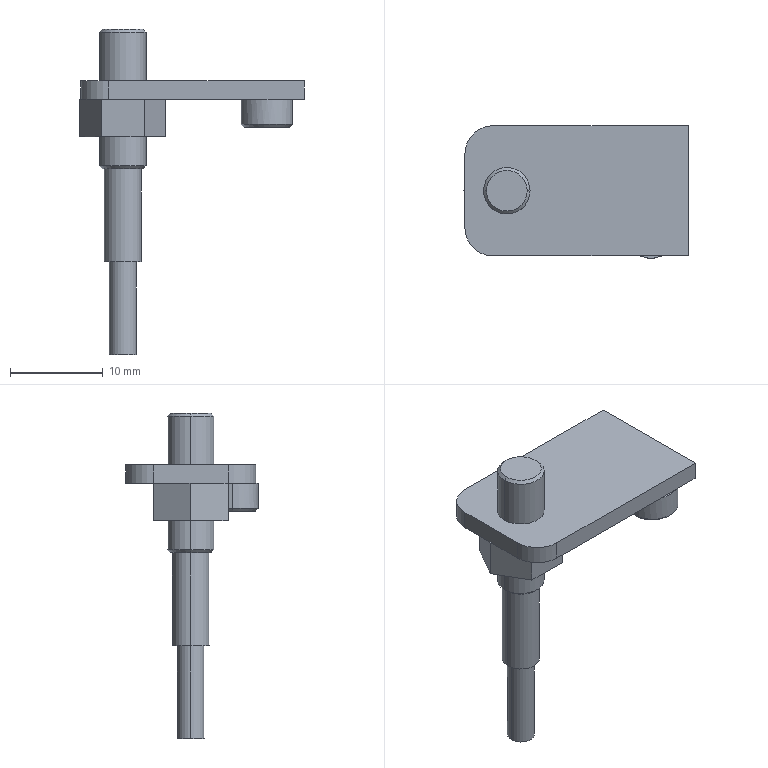Part | STEP file | 1105WWT4_1 | 1 solid | 45 faces | box 24.119 x 14.25 x 35 mm | volume 1315 mm3 | plane 27 | cylinder 12 | cone 6 | commonest cylinder face diameters 5 x4 2.9 x2 4 x2 5.5 x2 6 x2
STEP:
#1=CARTESIAN_POINT('',(-40.,-5.,-7.266));
#2=VERTEX_POINT('',#1);
#3=CARTESIAN_POINT('',(-35.,-5.,-7.266));
#4=VERTEX_POINT('',#3);
#5=CARTESIAN_POINT('',(-37.5,-5.,-7.266));
#6=DIRECTION('',(0.,0.,-1.));
#7=DIRECTION('',(-1.,0.,0.));
#8=AXIS2_PLACEMENT_3D('',#5,#6,#7);
#9=CIRCLE('',#8,2.5);
#10=EDGE_CURVE('',#2,#4,#9,.T.);
#11=ORIENTED_EDGE('',*,*,#10,.T.);
#12=CARTESIAN_POINT('',(-35.,-5.,-12.5));
#13=VERTEX_POINT('',#12);
#14=CARTESIAN_POINT('',(-35.,-5.,-14.46));
#15=DIRECTION('',(0.,0.,-1.));
#16=VECTOR('',#15,1000.);
#17=LINE('',#14,#16);
#18=EDGE_CURVE('',#4,#13,#17,.T.);
#19=ORIENTED_EDGE('',*,*,#18,.T.);
#20=CARTESIAN_POINT('',(-40.,-5.,-12.5));
#21=VERTEX_POINT('',#20);
#22=CARTESIAN_POINT('',(-37.5,-5.,-12.5));
#23=DIRECTION('',(0.,0.,-1.));
#24=DIRECTION('',(-1.,0.,0.));
#25=AXIS2_PLACEMENT_3D('',#22,#23,#24);
#26=CIRCLE('',#25,2.5);
#27=EDGE_CURVE('',#21,#13,#26,.T.);
#28=ORIENTED_EDGE('',*,*,#27,.F.);
#29=CARTESIAN_POINT('',(-40.,-5.,-14.46));
#30=DIRECTION('',(0.,0.,-1.));
#31=VECTOR('',#30,1000.);
#32=LINE('',#29,#31);
#33=EDGE_CURVE('',#2,#21,#32,.T.);
#34=ORIENTED_EDGE('',*,*,#33,.F.);
#35=EDGE_LOOP('',(#11,#19,#28,#34));
#36=FACE_OUTER_BOUND('',#35,.T.);
#37=CARTESIAN_POINT('',(-37.5,-5.,-14.46));
#38=DIRECTION('',(0.,0.,-1.));
#39=DIRECTION('',(-1.,0.,0.));
#40=AXIS2_PLACEMENT_3D('',#37,#38,#39);
#41=CYLINDRICAL_SURFACE('',#40,2.5);
#42=ADVANCED_FACE('',(#36),#41,.T.);
#43=CARTESIAN_POINT('',(-39.693,-5.,-6.96));
#44=VERTEX_POINT('',#43);
#45=CARTESIAN_POINT('',(-35.307,-5.,-6.96));
#46=VERTEX_POINT('',#45);
#47=CARTESIAN_POINT('',(-37.5,-5.,-6.96));
#48=DIRECTION('',(0.,0.,-1.));
#49=DIRECTION('',(-1.,0.,0.));
#50=AXIS2_PLACEMENT_3D('',#47,#48,#49);
#51=CIRCLE('',#50,2.193);
#52=EDGE_CURVE('',#44,#46,#51,.T.);
#53=ORIENTED_EDGE('',*,*,#52,.T.);
#54=CARTESIAN_POINT('',(-35.,-5.,-7.267));
#55=DIRECTION('',(0.7071,0.,-0.7071));
#56=VECTOR('',#55,1000.);
#57=LINE('',#54,#56);
#58=EDGE_CURVE('',#46,#4,#57,.T.);
#59=ORIENTED_EDGE('',*,*,#58,.T.);
#60=ORIENTED_EDGE('',*,*,#10,.F.);
#61=CARTESIAN_POINT('',(-40.,-5.,-7.267));
#62=DIRECTION('',(-0.7071,0.,-0.7071));
#63=VECTOR('',#62,1000.);
#64=LINE('',#61,#63);
#65=EDGE_CURVE('',#44,#2,#64,.T.);
#66=ORIENTED_EDGE('',*,*,#65,.F.);
#67=EDGE_LOOP('',(#53,#59,#60,#66));
#68=FACE_OUTER_BOUND('',#67,.T.);
#69=CARTESIAN_POINT('',(-37.5,-5.,-7.267));
#70=DIRECTION('',(0.,0.,-1.));
#71=DIRECTION('',(-1.,0.,0.));
#72=AXIS2_PLACEMENT_3D('',#69,#70,#71);
#73=CONICAL_SURFACE('',#72,2.5,0.7854);
#74=ADVANCED_FACE('',(#68),#73,.T.);
#75=CARTESIAN_POINT('',(-19.25,-9.5,-17.2));
#76=VERTEX_POINT('',#75);
#77=CARTESIAN_POINT('',(-24.75,-9.5,-17.2));
#78=VERTEX_POINT('',#77);
#79=CARTESIAN_POINT('',(-22.,-9.5,-17.2));
#80=DIRECTION('',(0.,0.,1.));
#81=DIRECTION('',(1.,0.,0.));
#82=AXIS2_PLACEMENT_3D('',#79,#80,#81);
#83=CIRCLE('',#82,2.75);
#84=EDGE_CURVE('',#76,#78,#83,.T.);
#85=ORIENTED_EDGE('',*,*,#84,.T.);
#86=CARTESIAN_POINT('',(-24.75,-9.5,-14.5));
#87=VERTEX_POINT('',#86);
#88=CARTESIAN_POINT('',(-24.75,-9.5,-15.85));
#89=DIRECTION('',(0.,0.,1.));
#90=VECTOR('',#89,1000.);
#91=LINE('',#88,#90);
#92=EDGE_CURVE('',#78,#87,#91,.T.);
#93=ORIENTED_EDGE('',*,*,#92,.T.);
#94=CARTESIAN_POINT('',(-19.25,-9.5,-14.5));
#95=VERTEX_POINT('',#94);
#96=CARTESIAN_POINT('',(-22.,-9.5,-14.5));
#97=DIRECTION('',(0.,0.,-1.));
#98=DIRECTION('',(1.,0.,0.));
#99=AXIS2_PLACEMENT_3D('',#96,#97,#98);
#100=CIRCLE('',#99,2.75);
#101=EDGE_CURVE('',#87,#95,#100,.T.);
#102=ORIENTED_EDGE('',*,*,#101,.T.);
#103=CARTESIAN_POINT('',(-19.25,-9.5,-15.85));
#104=DIRECTION('',(0.,0.,1.));
#105=VECTOR('',#104,1000.);
#106=LINE('',#103,#105);
#107=EDGE_CURVE('',#76,#95,#106,.T.);
#108=ORIENTED_EDGE('',*,*,#107,.F.);
#109=EDGE_LOOP('',(#85,#93,#102,#108));
#110=FACE_OUTER_BOUND('',#109,.T.);
#111=CARTESIAN_POINT('',(-22.,-9.5,-15.85));
#112=DIRECTION('',(0.,0.,1.));
#113=DIRECTION('',(1.,0.,0.));
#114=AXIS2_PLACEMENT_3D('',#111,#112,#113);
#115=CYLINDRICAL_SURFACE('',#114,2.75);
#116=ADVANCED_FACE('',(#110),#115,.T.);
#117=CARTESIAN_POINT('',(-19.55,-9.5,-17.5));
#118=VERTEX_POINT('',#117);
#119=CARTESIAN_POINT('',(-24.45,-9.5,-17.5));
#120=VERTEX_POINT('',#119);
#121=CARTESIAN_POINT('',(-22.,-9.5,-17.5));
#122=DIRECTION('',(0.,0.,1.));
#123=DIRECTION('',(1.,0.,0.));
#124=AXIS2_PLACEMENT_3D('',#121,#122,#123);
#125=CIRCLE('',#124,2.45);
#126=EDGE_CURVE('',#118,#120,#125,.T.);
#127=ORIENTED_EDGE('',*,*,#126,.T.);
#128=CARTESIAN_POINT('',(-24.75,-9.5,-17.2));
#129=DIRECTION('',(-0.7071,0.,0.7071));
#130=VECTOR('',#129,1000.);
#131=LINE('',#128,#130);
#132=EDGE_CURVE('',#120,#78,#131,.T.);
#133=ORIENTED_EDGE('',*,*,#132,.T.);
#134=ORIENTED_EDGE('',*,*,#84,.F.);
#135=CARTESIAN_POINT('',(-19.25,-9.5,-17.2));
#136=DIRECTION('',(0.7071,0.,0.7071));
#137=VECTOR('',#136,1000.);
#138=LINE('',#135,#137);
#139=EDGE_CURVE('',#118,#76,#138,.T.);
#140=ORIENTED_EDGE('',*,*,#139,.F.);
#141=EDGE_LOOP('',(#127,#133,#134,#140));
#142=FACE_OUTER_BOUND('',#141,.T.);
#143=CARTESIAN_POINT('',(-22.,-9.5,-17.2));
#144=DIRECTION('',(0.,0.,1.));
#145=DIRECTION('',(1.,0.,0.));
#146=AXIS2_PLACEMENT_3D('',#143,#144,#145);
#147=CONICAL_SURFACE('',#146,2.75,0.7854);
#148=ADVANCED_FACE('',(#142),#147,.T.);
#149=CARTESIAN_POINT('',(-40.,-5.,-18.5));
#150=VERTEX_POINT('',#149);
#151=CARTESIAN_POINT('',(-35.,-5.,-18.5));
#152=VERTEX_POINT('',#151);
#153=CARTESIAN_POINT('',(-37.5,-5.,-18.5));
#154=DIRECTION('',(0.,0.,-1.));
#155=DIRECTION('',(-1.,0.,0.));
#156=AXIS2_PLACEMENT_3D('',#153,#154,#155);
#157=CIRCLE('',#156,2.5);
#158=EDGE_CURVE('',#150,#152,#157,.T.);
#159=ORIENTED_EDGE('',*,*,#158,.T.);
#160=CARTESIAN_POINT('',(-35.,-5.,-21.654));
#161=VERTEX_POINT('',#160);
#162=CARTESIAN_POINT('',(-35.,-5.,-14.46));
#163=DIRECTION('',(0.,0.,-1.));
#164=VECTOR('',#163,1000.);
#165=LINE('',#162,#164);
#166=EDGE_CURVE('',#152,#161,#165,.T.);
#167=ORIENTED_EDGE('',*,*,#166,.T.);
#168=CARTESIAN_POINT('',(-40.,-5.,-21.654));
#169=VERTEX_POINT('',#168);
#170=CARTESIAN_POINT('',(-37.5,-5.,-21.654));
#171=DIRECTION('',(0.,0.,1.));
#172=DIRECTION('',(-1.,0.,0.));
#173=AXIS2_PLACEMENT_3D('',#170,#171,#172);
#174=CIRCLE('',#173,2.5);
#175=EDGE_CURVE('',#161,#169,#174,.T.);
#176=ORIENTED_EDGE('',*,*,#175,.T.);
#177=CARTESIAN_POINT('',(-40.,-5.,-14.46));
#178=DIRECTION('',(0.,0.,-1.));
#179=VECTOR('',#178,1000.);
#180=LINE('',#177,#179);
#181=EDGE_CURVE('',#150,#169,#180,.T.);
#182=ORIENTED_EDGE('',*,*,#181,.F.);
#183=EDGE_LOOP('',(#159,#167,#176,#182));
#184=FACE_OUTER_BOUND('',#183,.T.);
#185=CARTESIAN_POINT('',(-37.5,-5.,-14.46));
#186=DIRECTION('',(0.,0.,-1.));
#187=DIRECTION('',(-1.,0.,0.));
#188=AXIS2_PLACEMENT_3D('',#185,#186,#187);
#189=CYLINDRICAL_SURFACE('',#188,2.5);
#190=ADVANCED_FACE('',(#184),#189,.T.);
#191=CARTESIAN_POINT('',(-35.306,-5.,-21.96));
#192=VERTEX_POINT('',#191);
#193=CARTESIAN_POINT('',(-39.694,-5.,-21.96));
#194=VERTEX_POINT('',#193);
#195=CARTESIAN_POINT('',(-37.5,-5.,-21.96));
#196=DIRECTION('',(0.,0.,1.));
#197=DIRECTION('',(1.,0.,0.));
#198=AXIS2_PLACEMENT_3D('',#195,#196,#197);
#199=CIRCLE('',#198,2.194);
#200=EDGE_CURVE('',#192,#194,#199,.T.);
#201=ORIENTED_EDGE('',*,*,#200,.T.);
#202=CARTESIAN_POINT('',(-40.,-5.,-21.654));
#203=DIRECTION('',(-0.7071,0.,0.7071));
#204=VECTOR('',#203,1000.);
#205=LINE('',#202,#204);
#206=EDGE_CURVE('',#194,#169,#205,.T.);
#207=ORIENTED_EDGE('',*,*,#206,.T.);
#208=ORIENTED_EDGE('',*,*,#175,.F.);
#209=CARTESIAN_POINT('',(-35.,-5.,-21.654));
#210=DIRECTION('',(0.7071,0.,0.7071));
#211=VECTOR('',#210,1000.);
#212=LINE('',#209,#211);
#213=EDGE_CURVE('',#192,#161,#212,.T.);
#214=ORIENTED_EDGE('',*,*,#213,.F.);
#215=EDGE_LOOP('',(#201,#207,#208,#214));
#216=FACE_OUTER_BOUND('',#215,.T.);
#217=CARTESIAN_POINT('',(-37.5,-5.,-21.654));
#218=DIRECTION('',(0.,0.,1.));
#219=DIRECTION('',(1.,0.,0.));
#220=AXIS2_PLACEMENT_3D('',#217,#218,#219);
#221=CONICAL_SURFACE('',#220,2.5,0.7854);
#222=ADVANCED_FACE('',(#216),#221,.T.);
#223=CARTESIAN_POINT('',(-35.5,-5.,-21.96));
#224=VERTEX_POINT('',#223);
#225=CARTESIAN_POINT('',(-39.5,-5.,-21.96));
#226=VERTEX_POINT('',#225);
#227=CARTESIAN_POINT('',(-37.5,-5.,-21.96));
#228=DIRECTION('',(0.,0.,1.));
#229=DIRECTION('',(-1.,0.,0.));
#230=AXIS2_PLACEMENT_3D('',#227,#228,#229);
#231=CIRCLE('',#230,2.);
#232=EDGE_CURVE('',#224,#226,#231,.T.);
#233=ORIENTED_EDGE('',*,*,#232,.F.);
#234=CARTESIAN_POINT('',(-35.5,-5.,-31.96));
#235=VERTEX_POINT('',#234);
#236=CARTESIAN_POINT('',(-35.5,-5.,-26.96));
#237=DIRECTION('',(0.,0.,-1.));
#238=VECTOR('',#237,1000.);
#239=LINE('',#236,#238);
#240=EDGE_CURVE('',#224,#235,#239,.T.);
#241=ORIENTED_EDGE('',*,*,#240,.T.);
#242=CARTESIAN_POINT('',(-39.5,-5.,-31.96));
#243=VERTEX_POINT('',#242);
#244=CARTESIAN_POINT('',(-37.5,-5.,-31.96));
#245=DIRECTION('',(0.,0.,1.));
#246=DIRECTION('',(-1.,0.,0.));
#247=AXIS2_PLACEMENT_3D('',#244,#245,#246);
#248=CIRCLE('',#247,2.);
#249=EDGE_CURVE('',#235,#243,#248,.T.);
#250=ORIENTED_EDGE('',*,*,#249,.T.);
#251=CARTESIAN_POINT('',(-39.5,-5.,-26.96));
#252=DIRECTION('',(0.,0.,-1.));
#253=VECTOR('',#252,1000.);
#254=LINE('',#251,#253);
#255=EDGE_CURVE('',#226,#243,#254,.T.);
#256=ORIENTED_EDGE('',*,*,#255,.F.);
#257=EDGE_LOOP('',(#233,#241,#250,#256));
#258=FACE_OUTER_BOUND('',#257,.T.);
#259=CARTESIAN_POINT('',(-37.5,-5.,-26.96));
#260=DIRECTION('',(0.,0.,-1.));
#261=DIRECTION('',(-1.,0.,0.));
#262=AXIS2_PLACEMENT_3D('',#259,#260,#261);
#263=CYLINDRICAL_SURFACE('',#262,2.);
#264=ADVANCED_FACE('',(#258),#263,.T.);
#265=CARTESIAN_POINT('',(-36.05,-5.,-31.96));
#266=VERTEX_POINT('',#265);
#267=CARTESIAN_POINT('',(-38.95,-5.,-31.96));
#268=VERTEX_POINT('',#267);
#269=CARTESIAN_POINT('',(-37.5,-5.,-31.96));
#270=DIRECTION('',(0.,0.,1.));
#271=DIRECTION('',(-1.,0.,0.));
#272=AXIS2_PLACEMENT_3D('',#269,#270,#271);
#273=CIRCLE('',#272,1.45);
#274=EDGE_CURVE('',#266,#268,#273,.T.);
#275=ORIENTED_EDGE('',*,*,#274,.F.);
#276=CARTESIAN_POINT('',(-36.05,-5.,-41.96));
#277=VERTEX_POINT('',#276);
#278=CARTESIAN_POINT('',(-36.05,-5.,-36.96));
#279=DIRECTION('',(0.,0.,-1.));
#280=VECTOR('',#279,1000.);
#281=LINE('',#278,#280);
#282=EDGE_CURVE('',#266,#277,#281,.T.);
#283=ORIENTED_EDGE('',*,*,#282,.T.);
#284=CARTESIAN_POINT('',(-38.95,-5.,-41.96));
#285=VERTEX_POINT('',#284);
#286=CARTESIAN_POINT('',(-37.5,-5.,-41.96));
#287=DIRECTION('',(0.,0.,1.));
#288=DIRECTION('',(-1.,0.,0.));
#289=AXIS2_PLACEMENT_3D('',#286,#287,#288);
#290=CIRCLE('',#289,1.45);
#291=EDGE_CURVE('',#277,#285,#290,.T.);
#292=ORIENTED_EDGE('',*,*,#291,.T.);
#293=CARTESIAN_POINT('',(-38.95,-5.,-36.96));
#294=DIRECTION('',(0.,0.,-1.));
#295=VECTOR('',#294,1000.);
#296=LINE('',#293,#295);
#297=EDGE_CURVE('',#268,#285,#296,.T.);
#298=ORIENTED_EDGE('',*,*,#297,.F.);
#299=EDGE_LOOP('',(#275,#283,#292,#298));
#300=FACE_OUTER_BOUND('',#299,.T.);
#301=CARTESIAN_POINT('',(-37.5,-5.,-36.96));
#302=DIRECTION('',(0.,0.,-1.));
#303=DIRECTION('',(-1.,0.,0.));
#304=AXIS2_PLACEMENT_3D('',#301,#302,#303);
#305=CYLINDRICAL_SURFACE('',#304,1.45);
#306=ADVANCED_FACE('',(#300),#305,.T.);
#307=ORIENTED_EDGE('',*,*,#27,.T.);
#308=CARTESIAN_POINT('',(-37.5,-5.,-12.5));
#309=DIRECTION('',(0.,0.,-1.));
#310=DIRECTION('',(-1.,0.,0.));
#311=AXIS2_PLACEMENT_3D('',#308,#309,#310);
#312=CIRCLE('',#311,2.5);
#313=EDGE_CURVE('',#13,#21,#312,.T.);
#314=ORIENTED_EDGE('',*,*,#313,.T.);
#315=EDGE_LOOP('',(#307,#314));
#316=FACE_BOUND('',#315,.T.);
#317=CARTESIAN_POINT('',(-42.,-9.,-12.5));
#318=VERTEX_POINT('',#317);
#319=CARTESIAN_POINT('',(-39.,-12.,-12.5));
#320=VERTEX_POINT('',#319);
#321=CARTESIAN_POINT('',(-39.,-9.,-12.5));
#322=DIRECTION('',(0.,0.,1.));
#323=DIRECTION('',(1.,0.,0.));
#324=AXIS2_PLACEMENT_3D('',#321,#322,#323);
#325=CIRCLE('',#324,3.);
#326=EDGE_CURVE('',#318,#320,#325,.T.);
#327=ORIENTED_EDGE('',*,*,#326,.T.);
#328=CARTESIAN_POINT('',(-18.,-12.,-12.5));
#329=VERTEX_POINT('',#328);
#330=CARTESIAN_POINT('',(-37.5,-12.,-12.5));
#331=DIRECTION('',(1.,0.,0.));
#332=VECTOR('',#331,1000.);
#333=LINE('',#330,#332);
#334=EDGE_CURVE('',#320,#329,#333,.T.);
#335=ORIENTED_EDGE('',*,*,#334,.T.);
#336=CARTESIAN_POINT('',(-18.,2.,-12.5));
#337=VERTEX_POINT('',#336);
#338=CARTESIAN_POINT('',(-18.,-5.,-12.5));
#339=DIRECTION('',(0.,1.,0.));
#340=VECTOR('',#339,1000.);
#341=LINE('',#338,#340);
#342=EDGE_CURVE('',#329,#337,#341,.T.);
#343=ORIENTED_EDGE('',*,*,#342,.T.);
#344=CARTESIAN_POINT('',(-39.,2.,-12.5));
#345=VERTEX_POINT('',#344);
#346=CARTESIAN_POINT('',(-37.5,2.,-12.5));
#347=DIRECTION('',(-1.,0.,0.));
#348=VECTOR('',#347,1000.);
#349=LINE('',#346,#348);
#350=EDGE_CURVE('',#337,#345,#349,.T.);
#351=ORIENTED_EDGE('',*,*,#350,.T.);
#352=CARTESIAN_POINT('',(-42.,-1.,-12.5));
#353=VERTEX_POINT('',#352);
#354=CARTESIAN_POINT('',(-39.,-1.,-12.5));
#355=DIRECTION('',(0.,0.,1.));
#356=DIRECTION('',(1.,0.,0.));
#357=AXIS2_PLACEMENT_3D('',#354,#355,#356);
#358=CIRCLE('',#357,3.);
#359=EDGE_CURVE('',#345,#353,#358,.T.);
#360=ORIENTED_EDGE('',*,*,#359,.T.);
#361=CARTESIAN_POINT('',(-42.,-5.,-12.5));
#362=DIRECTION('',(0.,-1.,0.));
#363=VECTOR('',#362,1000.);
#364=LINE('',#361,#363);
#365=EDGE_CURVE('',#353,#318,#364,.T.);
#366=ORIENTED_EDGE('',*,*,#365,.T.);
#367=EDGE_LOOP('',(#327,#335,#343,#351,#360,#366));
#368=FACE_OUTER_BOUND('',#367,.T.);
#369=CARTESIAN_POINT('',(-37.5,-5.,-12.5));
#370=DIRECTION('',(0.,0.,1.));
#371=DIRECTION('',(1.,0.,0.));
#372=AXIS2_PLACEMENT_3D('',#369,#370,#371);
#373=PLANE('',#372);
#374=ADVANCED_FACE('',(#316,#368),#373,.T.);
#375=ORIENTED_EDGE('',*,*,#18,.F.);
#376=CARTESIAN_POINT('',(-37.5,-5.,-7.266));
#377=DIRECTION('',(0.,0.,-1.));
#378=DIRECTION('',(-1.,0.,0.));
#379=AXIS2_PLACEMENT_3D('',#376,#377,#378);
#380=CIRCLE('',#379,2.5);
#381=EDGE_CURVE('',#4,#2,#380,.T.);
#382=ORIENTED_EDGE('',*,*,#381,.T.);
#383=ORIENTED_EDGE('',*,*,#33,.T.);
#384=ORIENTED_EDGE('',*,*,#313,.F.);
#385=EDGE_LOOP('',(#375,#382,#383,#384));
#386=FACE_OUTER_BOUND('',#385,.T.);
#387=CARTESIAN_POINT('',(-37.5,-5.,-14.46));
#388=DIRECTION('',(0.,0.,-1.));
#389=DIRECTION('',(-1.,0.,0.));
#390=AXIS2_PLACEMENT_3D('',#387,#388,#389);
#391=CYLINDRICAL_SURFACE('',#390,2.5);
#392=ADVANCED_FACE('',(#386),#391,.T.);
#393=ORIENTED_EDGE('',*,*,#334,.F.);
#394=CARTESIAN_POINT('',(-39.,-12.,-14.5));
#395=VERTEX_POINT('',#394);
#396=CARTESIAN_POINT('',(-39.,-12.,-12.5));
#397=DIRECTION('',(0.,0.,-1.));
#398=VECTOR('',#397,1000.);
#399=LINE('',#396,#398);
#400=EDGE_CURVE('',#320,#395,#399,.T.);
#401=ORIENTED_EDGE('',*,*,#400,.T.);
#402=CARTESIAN_POINT('',(-23.146,-12.,-14.5));
#403=VERTEX_POINT('',#402);
#404=CARTESIAN_POINT('',(-39.,-12.,-14.5));
#405=DIRECTION('',(1.,0.,0.));
#406=VECTOR('',#405,1000.);
#407=LINE('',#404,#406);
#408=EDGE_CURVE('',#395,#403,#407,.T.);
#409=ORIENTED_EDGE('',*,*,#408,.T.);
#410=CARTESIAN_POINT('',(-20.854,-12.,-14.5));
#411=VERTEX_POINT('',#410);
#412=CARTESIAN_POINT('',(-39.,-12.,-14.5));
#413=DIRECTION('',(1.,0.,0.));
#414=VECTOR('',#413,1000.);
#415=LINE('',#412,#414);
#416=EDGE_CURVE('',#403,#411,#415,.T.);
#417=ORIENTED_EDGE('',*,*,#416,.T.);
#418=CARTESIAN_POINT('',(-18.,-12.,-14.5));
#419=VERTEX_POINT('',#418);
#420=CARTESIAN_POINT('',(-39.,-12.,-14.5));
#421=DIRECTION('',(1.,0.,0.));
#422=VECTOR('',#421,1000.);
#423=LINE('',#420,#422);
#424=EDGE_CURVE('',#411,#419,#423,.T.);
#425=ORIENTED_EDGE('',*,*,#424,.T.);
#426=CARTESIAN_POINT('',(-18.,-12.,-12.5));
#427=DIRECTION('',(0.,0.,1.));
#428=VECTOR('',#427,1000.);
#429=LINE('',#426,#428);
#430=EDGE_CURVE('',#419,#329,#429,.T.);
#431=ORIENTED_EDGE('',*,*,#430,.T.);
#432=EDGE_LOOP('',(#393,#401,#409,#417,#425,#431));
#433=FACE_OUTER_BOUND('',#432,.T.);
#434=CARTESIAN_POINT('',(-39.,-12.,-12.5));
#435=DIRECTION('',(0.,-1.,0.));
#436=DIRECTION('',(0.,0.,-1.));
#437=AXIS2_PLACEMENT_3D('',#434,#435,#436);
#438=PLANE('',#437);
#439=ADVANCED_FACE('',(#433),#438,.T.);
#440=ORIENTED_EDGE('',*,*,#326,.F.);
#441=CARTESIAN_POINT('',(-42.,-9.,-14.5));
#442=VERTEX_POINT('',#441);
#443=CARTESIAN_POINT('',(-42.,-9.,-12.5));
#444=DIRECTION('',(0.,0.,-1.));
#445=VECTOR('',#444,1000.);
#446=LINE('',#443,#445);
#447=EDGE_CURVE('',#318,#442,#446,.T.);
#448=ORIENTED_EDGE('',*,*,#447,.T.);
#449=CARTESIAN_POINT('',(-39.,-9.,-14.5));
#450=DIRECTION('',(0.,0.,1.));
#451=DIRECTION('',(1.,0.,0.));
#452=AXIS2_PLACEMENT_3D('',#449,#450,#451);
#453=CIRCLE('',#452,3.);
#454=EDGE_CURVE('',#442,#395,#453,.T.);
#455=ORIENTED_EDGE('',*,*,#454,.T.);
#456=ORIENTED_EDGE('',*,*,#400,.F.);
#457=EDGE_LOOP('',(#440,#448,#455,#456));
#458=FACE_OUTER_BOUND('',#457,.T.);
#459=CARTESIAN_POINT('',(-39.,-9.,-12.5));
#460=DIRECTION('',(0.,0.,1.));
#461=DIRECTION('',(1.,0.,0.));
#462=AXIS2_PLACEMENT_3D('',#459,#460,#461);
#463=CYLINDRICAL_SURFACE('',#462,3.);
#464=ADVANCED_FACE('',(#458),#463,.T.);
#465=ORIENTED_EDGE('',*,*,#365,.F.);
#466=CARTESIAN_POINT('',(-42.,-1.,-14.5));
#467=VERTEX_POINT('',#466);
#468=CARTESIAN_POINT('',(-42.,-1.,-12.5));
#469=DIRECTION('',(0.,0.,-1.));
#470=VECTOR('',#469,1000.);
#471=LINE('',#468,#470);
#472=EDGE_CURVE('',#353,#467,#471,.T.);
#473=ORIENTED_EDGE('',*,*,#472,.T.);
#474=CARTESIAN_POINT('',(-42.,-4.794,-14.5));
#475=VERTEX_POINT('',#474);
#476=CARTESIAN_POINT('',(-42.,-1.,-14.5));
#477=DIRECTION('',(0.,-1.,0.));
#478=VECTOR('',#477,1000.);
#479=LINE('',#476,#478);
#480=EDGE_CURVE('',#467,#475,#479,.T.);
#481=ORIENTED_EDGE('',*,*,#480,.T.);
#482=CARTESIAN_POINT('',(-42.,-5.206,-14.5));
#483=VERTEX_POINT('',#482);
#484=CARTESIAN_POINT('',(-42.,-1.,-14.5));
#485=DIRECTION('',(0.,-1.,0.));
#486=VECTOR('',#485,1000.);
#487=LINE('',#484,#486);
#488=EDGE_CURVE('',#475,#483,#487,.T.);
#489=ORIENTED_EDGE('',*,*,#488,.T.);
#490=CARTESIAN_POINT('',(-42.,-1.,-14.5));
#491=DIRECTION('',(0.,-1.,0.));
#492=VECTOR('',#491,1000.);
#493=LINE('',#490,#492);
#494=EDGE_CURVE('',#483,#442,#493,.T.);
#495=ORIENTED_EDGE('',*,*,#494,.T.);
#496=ORIENTED_EDGE('',*,*,#447,.F.);
#497=EDGE_LOOP('',(#465,#473,#481,#489,#495,#496));
#498=FACE_OUTER_BOUND('',#497,.T.);
#499=CARTESIAN_POINT('',(-42.,-1.,-12.5));
#500=DIRECTION('',(-1.,0.,0.));
#501=DIRECTION('',(0.,0.,1.));
#502=AXIS2_PLACEMENT_3D('',#499,#500,#501);
#503=PLANE('',#502);
#504=ADVANCED_FACE('',(#498),#503,.T.);
#505=ORIENTED_EDGE('',*,*,#359,.F.);
#506=CARTESIAN_POINT('',(-39.,2.,-14.5));
#507=VERTEX_POINT('',#506);
#508=CARTESIAN_POINT('',(-39.,2.,-12.5));
#509=DIRECTION('',(0.,0.,-1.));
#510=VECTOR('',#509,1000.);
#511=LINE('',#508,#510);
#512=EDGE_CURVE('',#345,#507,#511,.T.);
#513=ORIENTED_EDGE('',*,*,#512,.T.);
#514=CARTESIAN_POINT('',(-39.,-1.,-14.5));
#515=DIRECTION('',(0.,0.,1.));
#516=DIRECTION('',(1.,0.,0.));
#517=AXIS2_PLACEMENT_3D('',#514,#515,#516);
#518=CIRCLE('',#517,3.);
#519=EDGE_CURVE('',#507,#467,#518,.T.);
#520=ORIENTED_EDGE('',*,*,#519,.T.);
#521=ORIENTED_EDGE('',*,*,#472,.F.);
#522=EDGE_LOOP('',(#505,#513,#520,#521));
#523=FACE_OUTER_BOUND('',#522,.T.);
#524=CARTESIAN_POINT('',(-39.,-1.,-12.5));
#525=DIRECTION('',(0.,0.,1.));
#526=DIRECTION('',(1.,0.,0.));
#527=AXIS2_PLACEMENT_3D('',#524,#525,#526);
#528=CYLINDRICAL_SURFACE('',#527,3.);
#529=ADVANCED_FACE('',(#523),#528,.T.);
#530=ORIENTED_EDGE('',*,*,#350,.F.);
#531=CARTESIAN_POINT('',(-18.,2.,-14.5));
#532=VERTEX_POINT('',#531);
#533=CARTESIAN_POINT('',(-18.,2.,-12.5));
#534=DIRECTION('',(0.,0.,-1.));
#535=VECTOR('',#534,1000.);
#536=LINE('',#533,#535);
#537=EDGE_CURVE('',#337,#532,#536,.T.);
#538=ORIENTED_EDGE('',*,*,#537,.T.);
#539=CARTESIAN_POINT('',(-18.,2.,-14.5));
#540=DIRECTION('',(-1.,0.,0.));
#541=VECTOR('',#540,1000.);
#542=LINE('',#539,#541);
#543=EDGE_CURVE('',#532,#507,#542,.T.);
#544=ORIENTED_EDGE('',*,*,#543,.T.);
#545=ORIENTED_EDGE('',*,*,#512,.F.);
#546=EDGE_LOOP('',(#530,#538,#544,#545));
#547=FACE_OUTER_BOUND('',#546,.T.);
#548=CARTESIAN_POINT('',(-18.,2.,-12.5));
#549=DIRECTION('',(0.,1.,0.));
#550=DIRECTION('',(0.,0.,1.));
#551=AXIS2_PLACEMENT_3D('',#548,#549,#550);
#552=PLANE('',#551);
#553=ADVANCED_FACE('',(#547),#552,.T.);
#554=ORIENTED_EDGE('',*,*,#342,.F.);
#555=ORIENTED_EDGE('',*,*,#430,.F.);
#556=CARTESIAN_POINT('',(-18.,-12.,-14.5));
#557=DIRECTION('',(0.,1.,0.));
#558=VECTOR('',#557,1000.);
#559=LINE('',#556,#558);
#560=EDGE_CURVE('',#419,#532,#559,.T.);
#561=ORIENTED_EDGE('',*,*,#560,.T.);
#562=ORIENTED_EDGE('',*,*,#537,.F.);
#563=EDGE_LOOP('',(#554,#555,#561,#562));
#564=FACE_OUTER_BOUND('',#563,.T.);
#565=CARTESIAN_POINT('',(-18.,-12.,-12.5));
#566=DIRECTION('',(1.,0.,0.));
#567=DIRECTION('',(0.,0.,-1.));
#568=AXIS2_PLACEMENT_3D('',#565,#566,#567);
#569=PLANE('',#568);
#570=ADVANCED_FACE('',(#564),#569,.T.);
#571=ORIENTED_EDGE('',*,*,#58,.F.);
#572=CARTESIAN_POINT('',(-37.5,-5.,-6.96));
#573=DIRECTION('',(0.,0.,-1.));
#574=DIRECTION('',(-1.,0.,0.));
#575=AXIS2_PLACEMENT_3D('',#572,#573,#574);
#576=CIRCLE('',#575,2.193);
#577=EDGE_CURVE('',#46,#44,#576,.T.);
#578=ORIENTED_EDGE('',*,*,#577,.T.);
#579=ORIENTED_EDGE('',*,*,#65,.T.);
#580=ORIENTED_EDGE('',*,*,#381,.F.);
#581=EDGE_LOOP('',(#571,#578,#579,#580));
#582=FACE_OUTER_BOUND('',#581,.T.);
#583=CARTESIAN_POINT('',(-37.5,-5.,-7.267));
#584=DIRECTION('',(0.,0.,-1.));
#585=DIRECTION('',(-1.,0.,0.));
#586=AXIS2_PLACEMENT_3D('',#583,#584,#585);
#587=CONICAL_SURFACE('',#586,2.5,0.7854);
#588=ADVANCED_FACE('',(#582),#587,.T.);
#589=CARTESIAN_POINT('',(-22.,-9.5,-14.5));
#590=DIRECTION('',(0.,0.,-1.));
#591=DIRECTION('',(1.,0.,0.));
#592=AXIS2_PLACEMENT_3D('',#589,#590,#591);
#593=CIRCLE('',#592,2.75);
#594=EDGE_CURVE('',#403,#87,#593,.T.);
#595=ORIENTED_EDGE('',*,*,#594,.F.);
#596=ORIENTED_EDGE('',*,*,#408,.F.);
#597=ORIENTED_EDGE('',*,*,#454,.F.);
#598=ORIENTED_EDGE('',*,*,#494,.F.);
#599=CARTESIAN_POINT('',(-39.809,-9.,-14.5));
#600=VERTEX_POINT('',#599);
#601=CARTESIAN_POINT('',(-39.809,-9.,-14.5));
#602=DIRECTION('',(-0.5,0.866,0.));
#603=VECTOR('',#602,1000.);
#604=LINE('',#601,#603);
#605=EDGE_CURVE('',#600,#483,#604,.T.);
#606=ORIENTED_EDGE('',*,*,#605,.F.);
#607=CARTESIAN_POINT('',(-35.191,-9.,-14.5));
#608=VERTEX_POINT('',#607);
#609=CARTESIAN_POINT('',(-37.5,-9.,-14.5));
#610=DIRECTION('',(-1.,0.,0.));
#611=VECTOR('',#610,1000.);
#612=LINE('',#609,#611);
#613=EDGE_CURVE('',#608,#600,#612,.T.);
#614=ORIENTED_EDGE('',*,*,#613,.F.);
#615=CARTESIAN_POINT('',(-32.881,-5.,-14.5));
#616=VERTEX_POINT('',#615);
#617=CARTESIAN_POINT('',(-32.881,-5.,-14.5));
#618=DIRECTION('',(-0.5,-0.866,0.));
#619=VECTOR('',#618,1000.);
#620=LINE('',#617,#619);
#621=EDGE_CURVE('',#616,#608,#620,.T.);
#622=ORIENTED_EDGE('',*,*,#621,.F.);
#623=CARTESIAN_POINT('',(-35.191,-1.,-14.5));
#624=VERTEX_POINT('',#623);
#625=CARTESIAN_POINT('',(-35.191,-1.,-14.5));
#626=DIRECTION('',(0.5,-0.866,0.));
#627=VECTOR('',#626,1000.);
#628=LINE('',#625,#627);
#629=EDGE_CURVE('',#624,#616,#628,.T.);
#630=ORIENTED_EDGE('',*,*,#629,.F.);
#631=CARTESIAN_POINT('',(-39.809,-1.,-14.5));
#632=VERTEX_POINT('',#631);
#633=CARTESIAN_POINT('',(-37.5,-1.,-14.5));
#634=DIRECTION('',(1.,0.,0.));
#635=VECTOR('',#634,1000.);
#636=LINE('',#633,#635);
#637=EDGE_CURVE('',#632,#624,#636,.T.);
#638=ORIENTED_EDGE('',*,*,#637,.F.);
#639=CARTESIAN_POINT('',(-42.,-4.794,-14.5));
#640=DIRECTION('',(0.5,0.866,0.));
#641=VECTOR('',#640,1000.);
#642=LINE('',#639,#641);
#643=EDGE_CURVE('',#475,#632,#642,.T.);
#644=ORIENTED_EDGE('',*,*,#643,.F.);
#645=ORIENTED_EDGE('',*,*,#480,.F.);
#646=ORIENTED_EDGE('',*,*,#519,.F.);
#647=ORIENTED_EDGE('',*,*,#543,.F.);
#648=ORIENTED_EDGE('',*,*,#560,.F.);
#649=ORIENTED_EDGE('',*,*,#424,.F.);
#650=CARTESIAN_POINT('',(-22.,-9.5,-14.5));
#651=DIRECTION('',(0.,0.,-1.));
#652=DIRECTION('',(1.,0.,0.));
#653=AXIS2_PLACEMENT_3D('',#650,#651,#652);
#654=CIRCLE('',#653,2.75);
#655=EDGE_CURVE('',#95,#411,#654,.T.);
#656=ORIENTED_EDGE('',*,*,#655,.F.);
#657=ORIENTED_EDGE('',*,*,#101,.F.);
#658=EDGE_LOOP('',(#595,#596,#597,#598,#606,#614,#622,#630,#638,#644,#645,#646,#647,#648,#649,#656,#657));
#659=FACE_OUTER_BOUND('',#658,.T.);
#660=CARTESIAN_POINT('',(-37.5,-5.,-14.5));
#661=DIRECTION('',(0.,0.,1.));
#662=DIRECTION('',(1.,0.,0.));
#663=AXIS2_PLACEMENT_3D('',#660,#661,#662);
#664=PLANE('',#663);
#665=ADVANCED_FACE('',(#659),#664,.F.);
#666=ORIENTED_EDGE('',*,*,#416,.F.);
#667=CARTESIAN_POINT('',(-22.,-9.5,-14.5));
#668=DIRECTION('',(0.,0.,1.));
#669=DIRECTION('',(1.,0.,0.));
#670=AXIS2_PLACEMENT_3D('',#667,#668,#669);
#671=CIRCLE('',#670,2.75);
#672=EDGE_CURVE('',#403,#411,#671,.T.);
#673=ORIENTED_EDGE('',*,*,#672,.T.);
#674=EDGE_LOOP('',(#666,#673));
#675=FACE_OUTER_BOUND('',#674,.T.);
#676=CARTESIAN_POINT('',(-20.625,-9.5,-14.5));
#677=DIRECTION('',(0.,0.,1.));
#678=DIRECTION('',(1.,0.,0.));
#679=AXIS2_PLACEMENT_3D('',#676,#677,#678);
#680=PLANE('',#679);
#681=ADVANCED_FACE('',(#675),#680,.T.);
#682=CARTESIAN_POINT('',(-42.119,-5.,-14.5));
#683=VERTEX_POINT('',#682);
#684=CARTESIAN_POINT('',(-42.,-4.794,-14.5));
#685=DIRECTION('',(-0.5,-0.866,0.));
#686=VECTOR('',#685,1000.);
#687=LINE('',#684,#686);
#688=EDGE_CURVE('',#475,#683,#687,.T.);
#689=ORIENTED_EDGE('',*,*,#688,.T.);
#690=CARTESIAN_POINT('',(-42.119,-5.,-14.5));
#691=DIRECTION('',(0.5,-0.866,0.));
#692=VECTOR('',#691,1000.);
#693=LINE('',#690,#692);
#694=EDGE_CURVE('',#683,#483,#693,.T.);
#695=ORIENTED_EDGE('',*,*,#694,.T.);
#696=ORIENTED_EDGE('',*,*,#488,.F.);
#697=EDGE_LOOP('',(#689,#695,#696));
#698=FACE_OUTER_BOUND('',#697,.T.);
#699=CARTESIAN_POINT('',(-37.5,-5.,-14.5));
#700=DIRECTION('',(0.,0.,1.));
#701=DIRECTION('',(1.,0.,0.));
#702=AXIS2_PLACEMENT_3D('',#699,#700,#701);
#703=PLANE('',#702);
#704=ADVANCED_FACE('',(#698),#703,.T.);
#705=ORIENTED_EDGE('',*,*,#52,.F.);
#706=ORIENTED_EDGE('',*,*,#577,.F.);
#707=EDGE_LOOP('',(#705,#706));
#708=FACE_OUTER_BOUND('',#707,.T.);
#709=CARTESIAN_POINT('',(-38.597,-5.,-6.96));
#710=DIRECTION('',(0.,0.,1.));
#711=DIRECTION('',(1.,0.,0.));
#712=AXIS2_PLACEMENT_3D('',#709,#710,#711);
#713=PLANE('',#712);
#714=ADVANCED_FACE('',(#708),#713,.T.);
#715=ORIENTED_EDGE('',*,*,#92,.F.);
#716=CARTESIAN_POINT('',(-22.,-9.5,-17.2));
#717=DIRECTION('',(0.,0.,1.));
#718=DIRECTION('',(1.,0.,0.));
#719=AXIS2_PLACEMENT_3D('',#716,#717,#718);
#720=CIRCLE('',#719,2.75);
#721=EDGE_CURVE('',#78,#76,#720,.T.);
#722=ORIENTED_EDGE('',*,*,#721,.T.);
#723=ORIENTED_EDGE('',*,*,#107,.T.);
#724=ORIENTED_EDGE('',*,*,#655,.T.);
#725=ORIENTED_EDGE('',*,*,#672,.F.);
#726=ORIENTED_EDGE('',*,*,#594,.T.);
#727=EDGE_LOOP('',(#715,#722,#723,#724,#725,#726));
#728=FACE_OUTER_BOUND('',#727,.T.);
#729=CARTESIAN_POINT('',(-22.,-9.5,-15.85));
#730=DIRECTION('',(0.,0.,1.));
#731=DIRECTION('',(1.,0.,0.));
#732=AXIS2_PLACEMENT_3D('',#729,#730,#731);
#733=CYLINDRICAL_SURFACE('',#732,2.75);
#734=ADVANCED_FACE('',(#728),#733,.T.);
#735=ORIENTED_EDGE('',*,*,#694,.F.);
#736=CARTESIAN_POINT('',(-42.119,-5.,-18.5));
#737=VERTEX_POINT('',#736);
#738=CARTESIAN_POINT('',(-42.119,-5.,-14.5));
#739=DIRECTION('',(0.,0.,-1.));
#740=VECTOR('',#739,1000.);
#741=LINE('',#738,#740);
#742=EDGE_CURVE('',#683,#737,#741,.T.);
#743=ORIENTED_EDGE('',*,*,#742,.T.);
#744=CARTESIAN_POINT('',(-39.809,-9.,-18.5));
#745=VERTEX_POINT('',#744);
#746=CARTESIAN_POINT('',(-42.119,-5.,-18.5));
#747=DIRECTION('',(0.5,-0.866,0.));
#748=VECTOR('',#747,1000.);
#749=LINE('',#746,#748);
#750=EDGE_CURVE('',#737,#745,#749,.T.);
#751=ORIENTED_EDGE('',*,*,#750,.T.);
#752=CARTESIAN_POINT('',(-39.809,-9.,-14.5));
#753=DIRECTION('',(0.,0.,1.));
#754=VECTOR('',#753,1000.);
#755=LINE('',#752,#754);
#756=EDGE_CURVE('',#745,#600,#755,.T.);
#757=ORIENTED_EDGE('',*,*,#756,.T.);
#758=ORIENTED_EDGE('',*,*,#605,.T.);
#759=EDGE_LOOP('',(#735,#743,#751,#757,#758));
#760=FACE_OUTER_BOUND('',#759,.T.);
#761=CARTESIAN_POINT('',(-42.119,-5.,-14.5));
#762=DIRECTION('',(-0.866,-0.5,0.));
#763=DIRECTION('',(0.5,-0.866,0.));
#764=AXIS2_PLACEMENT_3D('',#761,#762,#763);
#765=PLANE('',#764);
#766=ADVANCED_FACE('',(#760),#765,.T.);
#767=ORIENTED_EDGE('',*,*,#613,.T.);
#768=ORIENTED_EDGE('',*,*,#756,.F.);
#769=CARTESIAN_POINT('',(-35.191,-9.,-18.5));
#770=VERTEX_POINT('',#769);
#771=CARTESIAN_POINT('',(-39.809,-9.,-18.5));
#772=DIRECTION('',(1.,0.,0.));
#773=VECTOR('',#772,1000.);
#774=LINE('',#771,#773);
#775=EDGE_CURVE('',#745,#770,#774,.T.);
#776=ORIENTED_EDGE('',*,*,#775,.T.);
#777=CARTESIAN_POINT('',(-35.191,-9.,-14.5));
#778=DIRECTION('',(0.,0.,1.));
#779=VECTOR('',#778,1000.);
#780=LINE('',#777,#779);
#781=EDGE_CURVE('',#770,#608,#780,.T.);
#782=ORIENTED_EDGE('',*,*,#781,.T.);
#783=EDGE_LOOP('',(#767,#768,#776,#782));
#784=FACE_OUTER_BOUND('',#783,.T.);
#785=CARTESIAN_POINT('',(-39.809,-9.,-14.5));
#786=DIRECTION('',(0.,-1.,0.));
#787=DIRECTION('',(0.,0.,-1.));
#788=AXIS2_PLACEMENT_3D('',#785,#786,#787);
#789=PLANE('',#788);
#790=ADVANCED_FACE('',(#784),#789,.T.);
#791=ORIENTED_EDGE('',*,*,#621,.T.);
#792=ORIENTED_EDGE('',*,*,#781,.F.);
#793=CARTESIAN_POINT('',(-32.881,-5.,-18.5));
#794=VERTEX_POINT('',#793);
#795=CARTESIAN_POINT('',(-35.191,-9.,-18.5));
#796=DIRECTION('',(0.5,0.866,0.));
#797=VECTOR('',#796,1000.);
#798=LINE('',#795,#797);
#799=EDGE_CURVE('',#770,#794,#798,.T.);
#800=ORIENTED_EDGE('',*,*,#799,.T.);
#801=CARTESIAN_POINT('',(-32.881,-5.,-14.5));
#802=DIRECTION('',(0.,0.,1.));
#803=VECTOR('',#802,1000.);
#804=LINE('',#801,#803);
#805=EDGE_CURVE('',#794,#616,#804,.T.);
#806=ORIENTED_EDGE('',*,*,#805,.T.);
#807=EDGE_LOOP('',(#791,#792,#800,#806));
#808=FACE_OUTER_BOUND('',#807,.T.);
#809=CARTESIAN_POINT('',(-35.191,-9.,-14.5));
#810=DIRECTION('',(0.866,-0.5,0.));
#811=DIRECTION('',(0.5,0.866,0.));
#812=AXIS2_PLACEMENT_3D('',#809,#810,#811);
#813=PLANE('',#812);
#814=ADVANCED_FACE('',(#808),#813,.T.);
#815=ORIENTED_EDGE('',*,*,#629,.T.);
#816=ORIENTED_EDGE('',*,*,#805,.F.);
#817=CARTESIAN_POINT('',(-35.191,-1.,-18.5));
#818=VERTEX_POINT('',#817);
#819=CARTESIAN_POINT('',(-32.881,-5.,-18.5));
#820=DIRECTION('',(-0.5,0.866,0.));
#821=VECTOR('',#820,1000.);
#822=LINE('',#819,#821);
#823=EDGE_CURVE('',#794,#818,#822,.T.);
#824=ORIENTED_EDGE('',*,*,#823,.T.);
#825=CARTESIAN_POINT('',(-35.191,-1.,-14.5));
#826=DIRECTION('',(0.,0.,1.));
#827=VECTOR('',#826,1000.);
#828=LINE('',#825,#827);
#829=EDGE_CURVE('',#818,#624,#828,.T.);
#830=ORIENTED_EDGE('',*,*,#829,.T.);
#831=EDGE_LOOP('',(#815,#816,#824,#830));
#832=FACE_OUTER_BOUND('',#831,.T.);
#833=CARTESIAN_POINT('',(-32.881,-5.,-14.5));
#834=DIRECTION('',(0.866,0.5,0.));
#835=DIRECTION('',(-0.5,0.866,0.));
#836=AXIS2_PLACEMENT_3D('',#833,#834,#835);
#837=PLANE('',#836);
#838=ADVANCED_FACE('',(#832),#837,.T.);
#839=ORIENTED_EDGE('',*,*,#637,.T.);
#840=ORIENTED_EDGE('',*,*,#829,.F.);
#841=CARTESIAN_POINT('',(-39.809,-1.,-18.5));
#842=VERTEX_POINT('',#841);
#843=CARTESIAN_POINT('',(-35.191,-1.,-18.5));
#844=DIRECTION('',(-1.,0.,0.));
#845=VECTOR('',#844,1000.);
#846=LINE('',#843,#845);
#847=EDGE_CURVE('',#818,#842,#846,.T.);
#848=ORIENTED_EDGE('',*,*,#847,.T.);
#849=CARTESIAN_POINT('',(-39.809,-1.,-14.5));
#850=DIRECTION('',(0.,0.,1.));
#851=VECTOR('',#850,1000.);
#852=LINE('',#849,#851);
#853=EDGE_CURVE('',#842,#632,#852,.T.);
#854=ORIENTED_EDGE('',*,*,#853,.T.);
#855=EDGE_LOOP('',(#839,#840,#848,#854));
#856=FACE_OUTER_BOUND('',#855,.T.);
#857=CARTESIAN_POINT('',(-35.191,-1.,-14.5));
#858=DIRECTION('',(0.,1.,0.));
#859=DIRECTION('',(0.,0.,1.));
#860=AXIS2_PLACEMENT_3D('',#857,#858,#859);
#861=PLANE('',#860);
#862=ADVANCED_FACE('',(#856),#861,.T.);
#863=ORIENTED_EDGE('',*,*,#643,.T.);
#864=ORIENTED_EDGE('',*,*,#853,.F.);
#865=CARTESIAN_POINT('',(-39.809,-1.,-18.5));
#866=DIRECTION('',(-0.5,-0.866,0.));
#867=VECTOR('',#866,1000.);
#868=LINE('',#865,#867);
#869=EDGE_CURVE('',#842,#737,#868,.T.);
#870=ORIENTED_EDGE('',*,*,#869,.T.);
#871=ORIENTED_EDGE('',*,*,#742,.F.);
#872=ORIENTED_EDGE('',*,*,#688,.F.);
#873=EDGE_LOOP('',(#863,#864,#870,#871,#872));
#874=FACE_OUTER_BOUND('',#873,.T.);
#875=CARTESIAN_POINT('',(-39.809,-1.,-14.5));
#876=DIRECTION('',(-0.866,0.5,0.));
#877=DIRECTION('',(-0.5,-0.866,0.));
#878=AXIS2_PLACEMENT_3D('',#875,#876,#877);
#879=PLANE('',#878);
#880=ADVANCED_FACE('',(#874),#879,.T.);
#881=ORIENTED_EDGE('',*,*,#132,.F.);
#882=CARTESIAN_POINT('',(-22.,-9.5,-17.5));
#883=DIRECTION('',(0.,0.,1.));
#884=DIRECTION('',(1.,0.,0.));
#885=AXIS2_PLACEMENT_3D('',#882,#883,#884);
#886=CIRCLE('',#885,2.45);
#887=EDGE_CURVE('',#120,#118,#886,.T.);
#888=ORIENTED_EDGE('',*,*,#887,.T.);
#889=ORIENTED_EDGE('',*,*,#139,.T.);
#890=ORIENTED_EDGE('',*,*,#721,.F.);
#891=EDGE_LOOP('',(#881,#888,#889,#890));
#892=FACE_OUTER_BOUND('',#891,.T.);
#893=CARTESIAN_POINT('',(-22.,-9.5,-17.2));
#894=DIRECTION('',(0.,0.,1.));
#895=DIRECTION('',(1.,0.,0.));
#896=AXIS2_PLACEMENT_3D('',#893,#894,#895);
#897=CONICAL_SURFACE('',#896,2.75,0.7854);
#898=ADVANCED_FACE('',(#892),#897,.T.);
#899=ORIENTED_EDGE('',*,*,#158,.F.);
#900=CARTESIAN_POINT('',(-37.5,-5.,-18.5));
#901=DIRECTION('',(0.,0.,-1.));
#902=DIRECTION('',(-1.,0.,0.));
#903=AXIS2_PLACEMENT_3D('',#900,#901,#902);
#904=CIRCLE('',#903,2.5);
#905=EDGE_CURVE('',#152,#150,#904,.T.);
#906=ORIENTED_EDGE('',*,*,#905,.F.);
#907=EDGE_LOOP('',(#899,#906));
#908=FACE_BOUND('',#907,.T.);
#909=ORIENTED_EDGE('',*,*,#775,.F.);
#910=ORIENTED_EDGE('',*,*,#750,.F.);
#911=ORIENTED_EDGE('',*,*,#869,.F.);
#912=ORIENTED_EDGE('',*,*,#847,.F.);
#913=ORIENTED_EDGE('',*,*,#823,.F.);
#914=ORIENTED_EDGE('',*,*,#799,.F.);
#915=EDGE_LOOP('',(#909,#910,#911,#912,#913,#914));
#916=FACE_OUTER_BOUND('',#915,.T.);
#917=CARTESIAN_POINT('',(-37.5,-5.,-18.5));
#918=DIRECTION('',(0.,0.,1.));
#919=DIRECTION('',(1.,0.,0.));
#920=AXIS2_PLACEMENT_3D('',#917,#918,#919);
#921=PLANE('',#920);
#922=ADVANCED_FACE('',(#908,#916),#921,.F.);
#923=ORIENTED_EDGE('',*,*,#126,.F.);
#924=ORIENTED_EDGE('',*,*,#887,.F.);
#925=EDGE_LOOP('',(#923,#924));
#926=FACE_OUTER_BOUND('',#925,.T.);
#927=CARTESIAN_POINT('',(-21.278,-8.25,-17.5));
#928=VERTEX_POINT('',#927);
#929=CARTESIAN_POINT('',(-22.722,-8.25,-17.5));
#930=VERTEX_POINT('',#929);
#931=CARTESIAN_POINT('',(-20.775,-8.25,-17.5));
#932=DIRECTION('',(-1.,0.,0.));
#933=VECTOR('',#932,1000.);
#934=LINE('',#931,#933);
#935=EDGE_CURVE('',#928,#930,#934,.T.);
#936=ORIENTED_EDGE('',*,*,#935,.T.);
#937=CARTESIAN_POINT('',(-23.443,-9.5,-17.5));
#938=VERTEX_POINT('',#937);
#939=CARTESIAN_POINT('',(-22.722,-8.25,-17.5));
#940=DIRECTION('',(-0.5,-0.866,0.));
#941=VECTOR('',#940,1000.);
#942=LINE('',#939,#941);
#943=EDGE_CURVE('',#930,#938,#942,.T.);
#944=ORIENTED_EDGE('',*,*,#943,.T.);
#945=CARTESIAN_POINT('',(-22.722,-10.75,-17.5));
#946=VERTEX_POINT('',#945);
#947=CARTESIAN_POINT('',(-23.443,-9.5,-17.5));
#948=DIRECTION('',(0.5,-0.866,0.));
#949=VECTOR('',#948,1000.);
#950=LINE('',#947,#949);
#951=EDGE_CURVE('',#938,#946,#950,.T.);
#952=ORIENTED_EDGE('',*,*,#951,.T.);
#953=CARTESIAN_POINT('',(-21.278,-10.75,-17.5));
#954=VERTEX_POINT('',#953);
#955=CARTESIAN_POINT('',(-20.775,-10.75,-17.5));
#956=DIRECTION('',(1.,0.,0.));
#957=VECTOR('',#956,1000.);
#958=LINE('',#955,#957);
#959=EDGE_CURVE('',#946,#954,#958,.T.);
#960=ORIENTED_EDGE('',*,*,#959,.T.);
#961=CARTESIAN_POINT('',(-20.557,-9.5,-17.5));
#962=VERTEX_POINT('',#961);
#963=CARTESIAN_POINT('',(-21.278,-10.75,-17.5));
#964=DIRECTION('',(0.5,0.866,0.));
#965=VECTOR('',#964,1000.);
#966=LINE('',#963,#965);
#967=EDGE_CURVE('',#954,#962,#966,.T.);
#968=ORIENTED_EDGE('',*,*,#967,.T.);
#969=CARTESIAN_POINT('',(-20.557,-9.5,-17.5));
#970=DIRECTION('',(-0.5,0.866,0.));
#971=VECTOR('',#970,1000.);
#972=LINE('',#969,#971);
#973=EDGE_CURVE('',#962,#928,#972,.T.);
#974=ORIENTED_EDGE('',*,*,#973,.T.);
#975=EDGE_LOOP('',(#936,#944,#952,#960,#968,#974));
#976=FACE_BOUND('',#975,.T.);
#977=CARTESIAN_POINT('',(-20.775,-9.5,-17.5));
#978=DIRECTION('',(0.,0.,-1.));
#979=DIRECTION('',(-1.,0.,0.));
#980=AXIS2_PLACEMENT_3D('',#977,#978,#979);
#981=PLANE('',#980);
#982=ADVANCED_FACE('',(#926,#976),#981,.T.);
#983=ORIENTED_EDGE('',*,*,#166,.F.);
#984=ORIENTED_EDGE('',*,*,#905,.T.);
#985=ORIENTED_EDGE('',*,*,#181,.T.);
#986=CARTESIAN_POINT('',(-37.5,-5.,-21.654));
#987=DIRECTION('',(0.,0.,1.));
#988=DIRECTION('',(-1.,0.,0.));
#989=AXIS2_PLACEMENT_3D('',#986,#987,#988);
#990=CIRCLE('',#989,2.5);
#991=EDGE_CURVE('',#169,#161,#990,.T.);
#992=ORIENTED_EDGE('',*,*,#991,.T.);
#993=EDGE_LOOP('',(#983,#984,#985,#992));
#994=FACE_OUTER_BOUND('',#993,.T.);
#995=CARTESIAN_POINT('',(-37.5,-5.,-14.46));
#996=DIRECTION('',(0.,0.,-1.));
#997=DIRECTION('',(-1.,0.,0.));
#998=AXIS2_PLACEMENT_3D('',#995,#996,#997);
#999=CYLINDRICAL_SURFACE('',#998,2.5);
#1000=ADVANCED_FACE('',(#994),#999,.T.);
#1001=CARTESIAN_POINT('',(-23.443,-9.5,-16.));
#1002=VERTEX_POINT('',#1001);
#1003=CARTESIAN_POINT('',(-23.443,-9.5,-17.5));
#1004=DIRECTION('',(0.,0.,1.));
#1005=VECTOR('',#1004,1000.);
#1006=LINE('',#1003,#1005);
#1007=EDGE_CURVE('',#938,#1002,#1006,.T.);
#1008=ORIENTED_EDGE('',*,*,#1007,.F.);
#1009=ORIENTED_EDGE('',*,*,#943,.F.);
#1010=CARTESIAN_POINT('',(-22.722,-8.25,-16.));
#1011=VERTEX_POINT('',#1010);
#1012=CARTESIAN_POINT('',(-22.722,-8.25,-17.5));
#1013=DIRECTION('',(0.,0.,-1.));
#1014=VECTOR('',#1013,1000.);
#1015=LINE('',#1012,#1014);
#1016=EDGE_CURVE('',#1011,#930,#1015,.T.);
#1017=ORIENTED_EDGE('',*,*,#1016,.F.);
#1018=CARTESIAN_POINT('',(-23.443,-9.5,-16.));
#1019=DIRECTION('',(0.5,0.866,0.));
#1020=VECTOR('',#1019,1000.);
#1021=LINE('',#1018,#1020);
#1022=EDGE_CURVE('',#1002,#1011,#1021,.T.);
#1023=ORIENTED_EDGE('',*,*,#1022,.F.);
#1024=EDGE_LOOP('',(#1008,#1009,#1017,#1023));
#1025=FACE_OUTER_BOUND('',#1024,.T.);
#1026=CARTESIAN_POINT('',(-23.443,-9.5,-17.5));
#1027=DIRECTION('',(-0.866,0.5,0.));
#1028=DIRECTION('',(-0.5,-0.866,0.));
#1029=AXIS2_PLACEMENT_3D('',#1026,#1027,#1028);
#1030=PLANE('',#1029);
#1031=ADVANCED_FACE('',(#1025),#1030,.F.);
#1032=ORIENTED_EDGE('',*,*,#1016,.T.);
#1033=ORIENTED_EDGE('',*,*,#935,.F.);
#1034=CARTESIAN_POINT('',(-21.278,-8.25,-16.));
#1035=VERTEX_POINT('',#1034);
#1036=CARTESIAN_POINT('',(-21.278,-8.25,-17.5));
#1037=DIRECTION('',(0.,0.,-1.));
#1038=VECTOR('',#1037,1000.);
#1039=LINE('',#1036,#1038);
#1040=EDGE_CURVE('',#1035,#928,#1039,.T.);
#1041=ORIENTED_EDGE('',*,*,#1040,.F.);
#1042=CARTESIAN_POINT('',(-22.722,-8.25,-16.));
#1043=DIRECTION('',(1.,0.,0.));
#1044=VECTOR('',#1043,1000.);
#1045=LINE('',#1042,#1044);
#1046=EDGE_CURVE('',#1011,#1035,#1045,.T.);
#1047=ORIENTED_EDGE('',*,*,#1046,.F.);
#1048=EDGE_LOOP('',(#1032,#1033,#1041,#1047));
#1049=FACE_OUTER_BOUND('',#1048,.T.);
#1050=CARTESIAN_POINT('',(-22.722,-8.25,-17.5));
#1051=DIRECTION('',(0.,1.,0.));
#1052=DIRECTION('',(0.,0.,1.));
#1053=AXIS2_PLACEMENT_3D('',#1050,#1051,#1052);
#1054=PLANE('',#1053);
#1055=ADVANCED_FACE('',(#1049),#1054,.F.);
#1056=ORIENTED_EDGE('',*,*,#1040,.T.);
#1057=ORIENTED_EDGE('',*,*,#973,.F.);
#1058=CARTESIAN_POINT('',(-20.557,-9.5,-16.));
#1059=VERTEX_POINT('',#1058);
#1060=CARTESIAN_POINT('',(-20.557,-9.5,-17.5));
#1061=DIRECTION('',(0.,0.,-1.));
#1062=VECTOR('',#1061,1000.);
#1063=LINE('',#1060,#1062);
#1064=EDGE_CURVE('',#1059,#962,#1063,.T.);
#1065=ORIENTED_EDGE('',*,*,#1064,.F.);
#1066=CARTESIAN_POINT('',(-21.278,-8.25,-16.));
#1067=DIRECTION('',(0.5,-0.866,0.));
#1068=VECTOR('',#1067,1000.);
#1069=LINE('',#1066,#1068);
#1070=EDGE_CURVE('',#1035,#1059,#1069,.T.);
#1071=ORIENTED_EDGE('',*,*,#1070,.F.);
#1072=EDGE_LOOP('',(#1056,#1057,#1065,#1071));
#1073=FACE_OUTER_BOUND('',#1072,.T.);
#1074=CARTESIAN_POINT('',(-21.278,-8.25,-17.5));
#1075=DIRECTION('',(0.866,0.5,0.));
#1076=DIRECTION('',(-0.5,0.866,0.));
#1077=AXIS2_PLACEMENT_3D('',#1074,#1075,#1076);
#1078=PLANE('',#1077);
#1079=ADVANCED_FACE('',(#1073),#1078,.F.);
#1080=ORIENTED_EDGE('',*,*,#1064,.T.);
#1081=ORIENTED_EDGE('',*,*,#967,.F.);
#1082=CARTESIAN_POINT('',(-21.278,-10.75,-16.));
#1083=VERTEX_POINT('',#1082);
#1084=CARTESIAN_POINT('',(-21.278,-10.75,-17.5));
#1085=DIRECTION('',(0.,0.,-1.));
#1086=VECTOR('',#1085,1000.);
#1087=LINE('',#1084,#1086);
#1088=EDGE_CURVE('',#1083,#954,#1087,.T.);
#1089=ORIENTED_EDGE('',*,*,#1088,.F.);
#1090=CARTESIAN_POINT('',(-20.557,-9.5,-16.));
#1091=DIRECTION('',(-0.5,-0.866,0.));
#1092=VECTOR('',#1091,1000.);
#1093=LINE('',#1090,#1092);
#1094=EDGE_CURVE('',#1059,#1083,#1093,.T.);
#1095=ORIENTED_EDGE('',*,*,#1094,.F.);
#1096=EDGE_LOOP('',(#1080,#1081,#1089,#1095));
#1097=FACE_OUTER_BOUND('',#1096,.T.);
#1098=CARTESIAN_POINT('',(-20.557,-9.5,-17.5));
#1099=DIRECTION('',(0.866,-0.5,0.));
#1100=DIRECTION('',(0.5,0.866,0.));
#1101=AXIS2_PLACEMENT_3D('',#1098,#1099,#1100);
#1102=PLANE('',#1101);
#1103=ADVANCED_FACE('',(#1097),#1102,.F.);
#1104=ORIENTED_EDGE('',*,*,#1088,.T.);
#1105=ORIENTED_EDGE('',*,*,#959,.F.);
#1106=CARTESIAN_POINT('',(-22.722,-10.75,-16.));
#1107=VERTEX_POINT('',#1106);
#1108=CARTESIAN_POINT('',(-22.722,-10.75,-17.5));
#1109=DIRECTION('',(0.,0.,-1.));
#1110=VECTOR('',#1109,1000.);
#1111=LINE('',#1108,#1110);
#1112=EDGE_CURVE('',#1107,#946,#1111,.T.);
#1113=ORIENTED_EDGE('',*,*,#1112,.F.);
#1114=CARTESIAN_POINT('',(-21.278,-10.75,-16.));
#1115=DIRECTION('',(-1.,0.,0.));
#1116=VECTOR('',#1115,1000.);
#1117=LINE('',#1114,#1116);
#1118=EDGE_CURVE('',#1083,#1107,#1117,.T.);
#1119=ORIENTED_EDGE('',*,*,#1118,.F.);
#1120=EDGE_LOOP('',(#1104,#1105,#1113,#1119));
#1121=FACE_OUTER_BOUND('',#1120,.T.);
#1122=CARTESIAN_POINT('',(-21.278,-10.75,-17.5));
#1123=DIRECTION('',(0.,-1.,0.));
#1124=DIRECTION('',(0.,0.,-1.));
#1125=AXIS2_PLACEMENT_3D('',#1122,#1123,#1124);
#1126=PLANE('',#1125);
#1127=ADVANCED_FACE('',(#1121),#1126,.F.);
#1128=ORIENTED_EDGE('',*,*,#1112,.T.);
#1129=ORIENTED_EDGE('',*,*,#951,.F.);
#1130=ORIENTED_EDGE('',*,*,#1007,.T.);
#1131=CARTESIAN_POINT('',(-22.722,-10.75,-16.));
#1132=DIRECTION('',(-0.5,0.866,0.));
#1133=VECTOR('',#1132,1000.);
#1134=LINE('',#1131,#1133);
#1135=EDGE_CURVE('',#1107,#1002,#1134,.T.);
#1136=ORIENTED_EDGE('',*,*,#1135,.F.);
#1137=EDGE_LOOP('',(#1128,#1129,#1130,#1136));
#1138=FACE_OUTER_BOUND('',#1137,.T.);
#1139=CARTESIAN_POINT('',(-22.722,-10.75,-17.5));
#1140=DIRECTION('',(-0.866,-0.5,0.));
#1141=DIRECTION('',(0.5,-0.866,0.));
#1142=AXIS2_PLACEMENT_3D('',#1139,#1140,#1141);
#1143=PLANE('',#1142);
#1144=ADVANCED_FACE('',(#1138),#1143,.F.);
#1145=ORIENTED_EDGE('',*,*,#206,.F.);
#1146=CARTESIAN_POINT('',(-37.5,-5.,-21.96));
#1147=DIRECTION('',(0.,0.,1.));
#1148=DIRECTION('',(1.,0.,0.));
#1149=AXIS2_PLACEMENT_3D('',#1146,#1147,#1148);
#1150=CIRCLE('',#1149,2.194);
#1151=EDGE_CURVE('',#194,#192,#1150,.T.);
#1152=ORIENTED_EDGE('',*,*,#1151,.T.);
#1153=ORIENTED_EDGE('',*,*,#213,.T.);
#1154=ORIENTED_EDGE('',*,*,#991,.F.);
#1155=EDGE_LOOP('',(#1145,#1152,#1153,#1154));
#1156=FACE_OUTER_BOUND('',#1155,.T.);
#1157=CARTESIAN_POINT('',(-37.5,-5.,-21.654));
#1158=DIRECTION('',(0.,0.,1.));
#1159=DIRECTION('',(1.,0.,0.));
#1160=AXIS2_PLACEMENT_3D('',#1157,#1158,#1159);
#1161=CONICAL_SURFACE('',#1160,2.5,0.7854);
#1162=ADVANCED_FACE('',(#1156),#1161,.T.);
#1163=ORIENTED_EDGE('',*,*,#1022,.T.);
#1164=ORIENTED_EDGE('',*,*,#1046,.T.);
#1165=ORIENTED_EDGE('',*,*,#1070,.T.);
#1166=ORIENTED_EDGE('',*,*,#1094,.T.);
#1167=ORIENTED_EDGE('',*,*,#1118,.T.);
#1168=ORIENTED_EDGE('',*,*,#1135,.T.);
#1169=EDGE_LOOP('',(#1163,#1164,#1165,#1166,#1167,#1168));
#1170=FACE_OUTER_BOUND('',#1169,.T.);
#1171=CARTESIAN_POINT('',(-37.5,-5.,-16.));
#1172=DIRECTION('',(0.,0.,1.));
#1173=DIRECTION('',(1.,0.,0.));
#1174=AXIS2_PLACEMENT_3D('',#1171,#1172,#1173);
#1175=PLANE('',#1174);
#1176=ADVANCED_FACE('',(#1170),#1175,.F.);
#1177=CARTESIAN_POINT('',(-37.5,-5.,-21.96));
#1178=DIRECTION('',(0.,0.,1.));
#1179=DIRECTION('',(-1.,0.,0.));
#1180=AXIS2_PLACEMENT_3D('',#1177,#1178,#1179);
#1181=CIRCLE('',#1180,2.);
#1182=EDGE_CURVE('',#226,#224,#1181,.T.);
#1183=ORIENTED_EDGE('',*,*,#1182,.T.);
#1184=ORIENTED_EDGE('',*,*,#232,.T.);
#1185=EDGE_LOOP('',(#1183,#1184));
#1186=FACE_BOUND('',#1185,.T.);
#1187=ORIENTED_EDGE('',*,*,#200,.F.);
#1188=ORIENTED_EDGE('',*,*,#1151,.F.);
#1189=EDGE_LOOP('',(#1187,#1188));
#1190=FACE_OUTER_BOUND('',#1189,.T.);
#1191=CARTESIAN_POINT('',(-39.597,-5.,-21.96));
#1192=DIRECTION('',(0.,0.,-1.));
#1193=DIRECTION('',(-1.,0.,0.));
#1194=AXIS2_PLACEMENT_3D('',#1191,#1192,#1193);
#1195=PLANE('',#1194);
#1196=ADVANCED_FACE('',(#1186,#1190),#1195,.T.);
#1197=ORIENTED_EDGE('',*,*,#240,.F.);
#1198=ORIENTED_EDGE('',*,*,#1182,.F.);
#1199=ORIENTED_EDGE('',*,*,#255,.T.);
#1200=CARTESIAN_POINT('',(-37.5,-5.,-31.96));
#1201=DIRECTION('',(0.,0.,1.));
#1202=DIRECTION('',(-1.,0.,0.));
#1203=AXIS2_PLACEMENT_3D('',#1200,#1201,#1202);
#1204=CIRCLE('',#1203,2.);
#1205=EDGE_CURVE('',#243,#235,#1204,.T.);
#1206=ORIENTED_EDGE('',*,*,#1205,.T.);
#1207=EDGE_LOOP('',(#1197,#1198,#1199,#1206));
#1208=FACE_OUTER_BOUND('',#1207,.T.);
#1209=CARTESIAN_POINT('',(-37.5,-5.,-26.96));
#1210=DIRECTION('',(0.,0.,-1.));
#1211=DIRECTION('',(-1.,0.,0.));
#1212=AXIS2_PLACEMENT_3D('',#1209,#1210,#1211);
#1213=CYLINDRICAL_SURFACE('',#1212,2.);
#1214=ADVANCED_FACE('',(#1208),#1213,.T.);
#1215=CARTESIAN_POINT('',(-37.5,-5.,-31.96));
#1216=DIRECTION('',(0.,0.,1.));
#1217=DIRECTION('',(-1.,0.,0.));
#1218=AXIS2_PLACEMENT_3D('',#1215,#1216,#1217);
#1219=CIRCLE('',#1218,1.45);
#1220=EDGE_CURVE('',#268,#266,#1219,.T.);
#1221=ORIENTED_EDGE('',*,*,#1220,.T.);
#1222=ORIENTED_EDGE('',*,*,#274,.T.);
#1223=EDGE_LOOP('',(#1221,#1222));
#1224=FACE_BOUND('',#1223,.T.);
#1225=ORIENTED_EDGE('',*,*,#1205,.F.);
#1226=ORIENTED_EDGE('',*,*,#249,.F.);
#1227=EDGE_LOOP('',(#1225,#1226));
#1228=FACE_OUTER_BOUND('',#1227,.T.);
#1229=CARTESIAN_POINT('',(-39.225,-5.,-31.96));
#1230=DIRECTION('',(0.,0.,-1.));
#1231=DIRECTION('',(-1.,0.,0.));
#1232=AXIS2_PLACEMENT_3D('',#1229,#1230,#1231);
#1233=PLANE('',#1232);
#1234=ADVANCED_FACE('',(#1224,#1228),#1233,.T.);
#1235=ORIENTED_EDGE('',*,*,#282,.F.);
#1236=ORIENTED_EDGE('',*,*,#1220,.F.);
#1237=ORIENTED_EDGE('',*,*,#297,.T.);
#1238=CARTESIAN_POINT('',(-37.5,-5.,-41.96));
#1239=DIRECTION('',(0.,0.,1.));
#1240=DIRECTION('',(-1.,0.,0.));
#1241=AXIS2_PLACEMENT_3D('',#1238,#1239,#1240);
#1242=CIRCLE('',#1241,1.45);
#1243=EDGE_CURVE('',#285,#277,#1242,.T.);
#1244=ORIENTED_EDGE('',*,*,#1243,.T.);
#1245=EDGE_LOOP('',(#1235,#1236,#1237,#1244));
#1246=FACE_OUTER_BOUND('',#1245,.T.);
#1247=CARTESIAN_POINT('',(-37.5,-5.,-36.96));
#1248=DIRECTION('',(0.,0.,-1.));
#1249=DIRECTION('',(-1.,0.,0.));
#1250=AXIS2_PLACEMENT_3D('',#1247,#1248,#1249);
#1251=CYLINDRICAL_SURFACE('',#1250,1.45);
#1252=ADVANCED_FACE('',(#1246),#1251,.T.);
#1253=ORIENTED_EDGE('',*,*,#1243,.F.);
#1254=ORIENTED_EDGE('',*,*,#291,.F.);
#1255=EDGE_LOOP('',(#1253,#1254));
#1256=FACE_OUTER_BOUND('',#1255,.T.);
#1257=CARTESIAN_POINT('',(-38.225,-5.,-41.96));
#1258=DIRECTION('',(0.,0.,-1.));
#1259=DIRECTION('',(-1.,0.,0.));
#1260=AXIS2_PLACEMENT_3D('',#1257,#1258,#1259);
#1261=PLANE('',#1260);
#1262=ADVANCED_FACE('',(#1256),#1261,.T.);
#1263=CLOSED_SHELL('',(#42,#74,#116,#148,#190,#222,#264,#306,#374,#392,#439,#464,#504,#529,#553,#570,#588,#665,#681,#704,#714,#734,#766,#790,#814,#838,#862,#880,#898,#922,#982,#1000,#1031,#1055,#1079,#1103,#1127,#1144,#1162,#1176,#1196,#1214,#1234,#1252,#1262));
#1264=MANIFOLD_SOLID_BREP('',#1263);
#1265=CARTESIAN_POINT('',(0.,0.,0.));
#1266=DIRECTION('',(0.,0.,1.));
#1267=DIRECTION('',(1.,0.,0.));
#1268=AXIS2_PLACEMENT_3D('',#1265,#1266,#1267);
#1269=(LENGTH_UNIT()NAMED_UNIT(*)SI_UNIT(.MILLI.,.METRE.));
#1270=UNCERTAINTY_MEASURE_WITH_UNIT(LENGTH_MEASURE(0.00001),#1269,'','');
#1271=(NAMED_UNIT(*)PLANE_ANGLE_UNIT()SI_UNIT($,.RADIAN.));
#1272=(NAMED_UNIT(*)SI_UNIT($,.STERADIAN.)SOLID_ANGLE_UNIT());
#1273=(GEOMETRIC_REPRESENTATION_CONTEXT(3)GLOBAL_UNCERTAINTY_ASSIGNED_CONTEXT((#1270))GLOBAL_UNIT_ASSIGNED_CONTEXT((#1269,#1271,#1272))REPRESENTATION_CONTEXT('',''));
#1274=ADVANCED_BREP_SHAPE_REPRESENTATION('',(#1264,#1268),#1273);